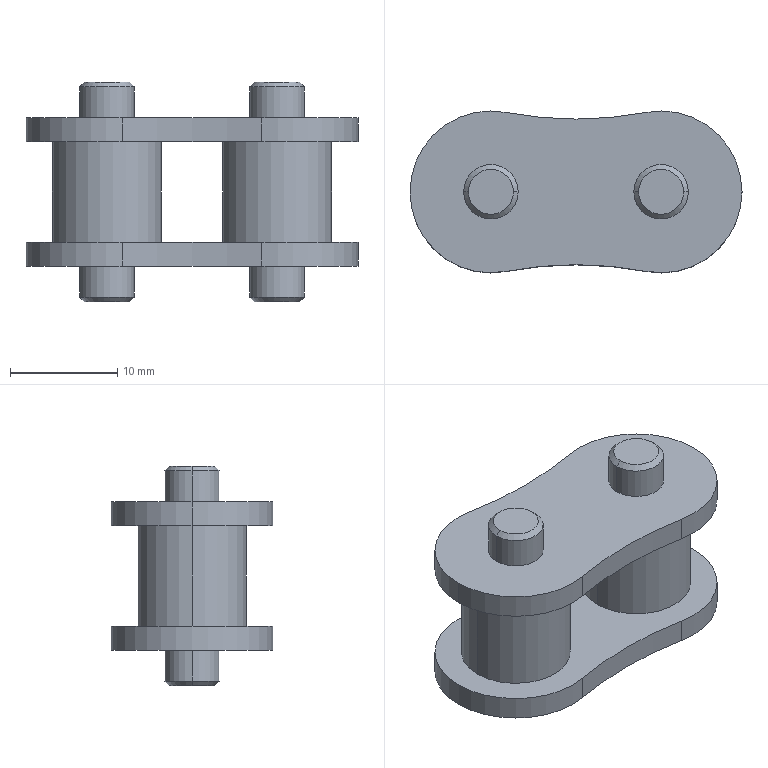Part | NX | features BREP 1 | 1 solid | 38 faces | box 30.965 x 15.09 x 20.5 mm | volume 3582 mm3 | cylinder 22 | cone 8 | plane 8 | commonest cylinder face diameters 5.09 x8 15.09 x6 10.16 x4 69.169 x4
STEP:
#1=CARTESIAN_POINT('',(-10.039,0.,-10.25));
#2=VERTEX_POINT('',#1);
#3=CARTESIAN_POINT('',(-5.837,0.,-10.25));
#4=VERTEX_POINT('',#3);
#5=CARTESIAN_POINT('',(-7.938,0.,-10.25));
#6=DIRECTION('',(0.,0.,-1.));
#7=DIRECTION('',(-1.,0.,0.));
#8=AXIS2_PLACEMENT_3D('',#5,#6,#7);
#9=CIRCLE('',#8,2.101);
#10=EDGE_CURVE('',#2,#4,#9,.T.);
#11=ORIENTED_EDGE('',*,*,#10,.F.);
#12=CARTESIAN_POINT('',(-10.482,0.,-9.806));
#13=VERTEX_POINT('',#12);
#14=CARTESIAN_POINT('',(-10.482,0.,-9.806));
#15=DIRECTION('',(-0.7071,0.,0.7071));
#16=VECTOR('',#15,1000.);
#17=LINE('',#14,#16);
#18=EDGE_CURVE('',#13,#2,#17,.F.);
#19=ORIENTED_EDGE('',*,*,#18,.F.);
#20=CARTESIAN_POINT('',(-5.393,0.,-9.806));
#21=VERTEX_POINT('',#20);
#22=CARTESIAN_POINT('',(-7.938,0.,-9.806));
#23=DIRECTION('',(0.,0.,1.));
#24=DIRECTION('',(-1.,0.,0.));
#25=AXIS2_PLACEMENT_3D('',#22,#23,#24);
#26=CIRCLE('',#25,2.545);
#27=EDGE_CURVE('',#21,#13,#26,.T.);
#28=ORIENTED_EDGE('',*,*,#27,.F.);
#29=CARTESIAN_POINT('',(-5.393,0.,-9.806));
#30=DIRECTION('',(0.7071,0.,0.7071));
#31=VECTOR('',#30,1000.);
#32=LINE('',#29,#31);
#33=EDGE_CURVE('',#21,#4,#32,.F.);
#34=ORIENTED_EDGE('',*,*,#33,.T.);
#35=EDGE_LOOP('',(#11,#19,#28,#34));
#36=FACE_BOUND('',#35,.T.);
#37=CARTESIAN_POINT('',(-7.938,0.,-9.806));
#38=DIRECTION('',(0.,0.,1.));
#39=DIRECTION('',(1.,0.,0.));
#40=AXIS2_PLACEMENT_3D('',#37,#38,#39);
#41=CONICAL_SURFACE('',#40,2.545,0.7854);
#42=ADVANCED_FACE('',(#36),#41,.T.);
#43=CARTESIAN_POINT('',(5.837,0.,-10.25));
#44=VERTEX_POINT('',#43);
#45=CARTESIAN_POINT('',(10.039,0.,-10.25));
#46=VERTEX_POINT('',#45);
#47=CARTESIAN_POINT('',(7.938,0.,-10.25));
#48=DIRECTION('',(0.,0.,-1.));
#49=DIRECTION('',(-1.,0.,0.));
#50=AXIS2_PLACEMENT_3D('',#47,#48,#49);
#51=CIRCLE('',#50,2.101);
#52=EDGE_CURVE('',#44,#46,#51,.T.);
#53=ORIENTED_EDGE('',*,*,#52,.F.);
#54=CARTESIAN_POINT('',(5.393,0.,-9.806));
#55=VERTEX_POINT('',#54);
#56=CARTESIAN_POINT('',(5.393,0.,-9.806));
#57=DIRECTION('',(-0.7071,0.,0.7071));
#58=VECTOR('',#57,1000.);
#59=LINE('',#56,#58);
#60=EDGE_CURVE('',#55,#44,#59,.F.);
#61=ORIENTED_EDGE('',*,*,#60,.F.);
#62=CARTESIAN_POINT('',(10.482,0.,-9.806));
#63=VERTEX_POINT('',#62);
#64=CARTESIAN_POINT('',(7.938,0.,-9.806));
#65=DIRECTION('',(0.,0.,1.));
#66=DIRECTION('',(-1.,0.,0.));
#67=AXIS2_PLACEMENT_3D('',#64,#65,#66);
#68=CIRCLE('',#67,2.545);
#69=EDGE_CURVE('',#63,#55,#68,.T.);
#70=ORIENTED_EDGE('',*,*,#69,.F.);
#71=CARTESIAN_POINT('',(10.482,0.,-9.806));
#72=DIRECTION('',(0.7071,0.,0.7071));
#73=VECTOR('',#72,1000.);
#74=LINE('',#71,#73);
#75=EDGE_CURVE('',#63,#46,#74,.F.);
#76=ORIENTED_EDGE('',*,*,#75,.T.);
#77=EDGE_LOOP('',(#53,#61,#70,#76));
#78=FACE_BOUND('',#77,.T.);
#79=CARTESIAN_POINT('',(7.938,0.,-9.806));
#80=DIRECTION('',(0.,0.,1.));
#81=DIRECTION('',(1.,0.,0.));
#82=AXIS2_PLACEMENT_3D('',#79,#80,#81);
#83=CONICAL_SURFACE('',#82,2.545,0.7854);
#84=ADVANCED_FACE('',(#78),#83,.T.);
#85=ORIENTED_EDGE('',*,*,#27,.T.);
#86=CARTESIAN_POINT('',(-10.482,0.,-6.92));
#87=VERTEX_POINT('',#86);
#88=CARTESIAN_POINT('',(-10.482,0.,-10.25));
#89=DIRECTION('',(0.,0.,1.));
#90=VECTOR('',#89,1000.);
#91=LINE('',#88,#90);
#92=EDGE_CURVE('',#87,#13,#91,.F.);
#93=ORIENTED_EDGE('',*,*,#92,.F.);
#94=CARTESIAN_POINT('',(-5.393,0.,-6.92));
#95=VERTEX_POINT('',#94);
#96=CARTESIAN_POINT('',(-7.938,0.,-6.92));
#97=DIRECTION('',(0.,0.,-1.));
#98=DIRECTION('',(-1.,0.,0.));
#99=AXIS2_PLACEMENT_3D('',#96,#97,#98);
#100=CIRCLE('',#99,2.545);
#101=EDGE_CURVE('',#87,#95,#100,.T.);
#102=ORIENTED_EDGE('',*,*,#101,.T.);
#103=CARTESIAN_POINT('',(-5.393,0.,-10.25));
#104=DIRECTION('',(0.,0.,1.));
#105=VECTOR('',#104,1000.);
#106=LINE('',#103,#105);
#107=EDGE_CURVE('',#95,#21,#106,.F.);
#108=ORIENTED_EDGE('',*,*,#107,.T.);
#109=EDGE_LOOP('',(#85,#93,#102,#108));
#110=FACE_BOUND('',#109,.T.);
#111=CARTESIAN_POINT('',(-7.938,0.,-10.25));
#112=DIRECTION('',(0.,0.,1.));
#113=DIRECTION('',(1.,0.,0.));
#114=AXIS2_PLACEMENT_3D('',#111,#112,#113);
#115=CYLINDRICAL_SURFACE('',#114,2.545);
#116=ADVANCED_FACE('',(#110),#115,.T.);
#117=ORIENTED_EDGE('',*,*,#69,.T.);
#118=CARTESIAN_POINT('',(5.393,0.,-6.92));
#119=VERTEX_POINT('',#118);
#120=CARTESIAN_POINT('',(5.393,0.,-10.25));
#121=DIRECTION('',(0.,0.,1.));
#122=VECTOR('',#121,1000.);
#123=LINE('',#120,#122);
#124=EDGE_CURVE('',#119,#55,#123,.F.);
#125=ORIENTED_EDGE('',*,*,#124,.F.);
#126=CARTESIAN_POINT('',(10.482,0.,-6.92));
#127=VERTEX_POINT('',#126);
#128=CARTESIAN_POINT('',(7.938,0.,-6.92));
#129=DIRECTION('',(0.,0.,-1.));
#130=DIRECTION('',(-1.,0.,0.));
#131=AXIS2_PLACEMENT_3D('',#128,#129,#130);
#132=CIRCLE('',#131,2.545);
#133=EDGE_CURVE('',#119,#127,#132,.T.);
#134=ORIENTED_EDGE('',*,*,#133,.T.);
#135=CARTESIAN_POINT('',(10.482,0.,-10.25));
#136=DIRECTION('',(0.,0.,1.));
#137=VECTOR('',#136,1000.);
#138=LINE('',#135,#137);
#139=EDGE_CURVE('',#127,#63,#138,.F.);
#140=ORIENTED_EDGE('',*,*,#139,.T.);
#141=EDGE_LOOP('',(#117,#125,#134,#140));
#142=FACE_BOUND('',#141,.T.);
#143=CARTESIAN_POINT('',(7.938,0.,-10.25));
#144=DIRECTION('',(0.,0.,1.));
#145=DIRECTION('',(1.,0.,0.));
#146=AXIS2_PLACEMENT_3D('',#143,#144,#145);
#147=CYLINDRICAL_SURFACE('',#146,2.545);
#148=ADVANCED_FACE('',(#142),#147,.T.);
#149=CARTESIAN_POINT('',(6.516,-7.41,-6.92));
#150=VERTEX_POINT('',#149);
#151=CARTESIAN_POINT('',(15.482,0.,-6.92));
#152=VERTEX_POINT('',#151);
#153=CARTESIAN_POINT('',(7.938,0.,-6.92));
#154=DIRECTION('',(0.,0.,1.));
#155=DIRECTION('',(1.,0.,0.));
#156=AXIS2_PLACEMENT_3D('',#153,#154,#155);
#157=CIRCLE('',#156,7.545);
#158=EDGE_CURVE('',#150,#152,#157,.T.);
#159=ORIENTED_EDGE('',*,*,#158,.T.);
#160=CARTESIAN_POINT('',(15.482,0.,-4.7));
#161=VERTEX_POINT('',#160);
#162=CARTESIAN_POINT('',(15.482,0.,-6.92));
#163=DIRECTION('',(0.,0.,1.));
#164=VECTOR('',#163,1000.);
#165=LINE('',#162,#164);
#166=EDGE_CURVE('',#152,#161,#165,.T.);
#167=ORIENTED_EDGE('',*,*,#166,.T.);
#168=CARTESIAN_POINT('',(6.516,-7.41,-4.7));
#169=VERTEX_POINT('',#168);
#170=CARTESIAN_POINT('',(7.938,0.,-4.7));
#171=DIRECTION('',(0.,0.,1.));
#172=DIRECTION('',(1.,0.,0.));
#173=AXIS2_PLACEMENT_3D('',#170,#171,#172);
#174=CIRCLE('',#173,7.545);
#175=EDGE_CURVE('',#169,#161,#174,.T.);
#176=ORIENTED_EDGE('',*,*,#175,.F.);
#177=CARTESIAN_POINT('',(6.516,-7.41,-6.92));
#178=DIRECTION('',(0.,0.,1.));
#179=VECTOR('',#178,1000.);
#180=LINE('',#177,#179);
#181=EDGE_CURVE('',#150,#169,#180,.T.);
#182=ORIENTED_EDGE('',*,*,#181,.F.);
#183=EDGE_LOOP('',(#159,#167,#176,#182));
#184=FACE_BOUND('',#183,.T.);
#185=CARTESIAN_POINT('',(7.938,0.,-6.92));
#186=DIRECTION('',(0.,0.,1.));
#187=DIRECTION('',(1.,0.,0.));
#188=AXIS2_PLACEMENT_3D('',#185,#186,#187);
#189=CYLINDRICAL_SURFACE('',#188,7.545);
#190=ADVANCED_FACE('',(#184),#189,.T.);
#191=CARTESIAN_POINT('',(-5.837,0.,10.25));
#192=VERTEX_POINT('',#191);
#193=CARTESIAN_POINT('',(-10.039,0.,10.25));
#194=VERTEX_POINT('',#193);
#195=CARTESIAN_POINT('',(-7.938,0.,10.25));
#196=DIRECTION('',(0.,0.,1.));
#197=DIRECTION('',(1.,0.,0.));
#198=AXIS2_PLACEMENT_3D('',#195,#196,#197);
#199=CIRCLE('',#198,2.101);
#200=EDGE_CURVE('',#192,#194,#199,.T.);
#201=ORIENTED_EDGE('',*,*,#200,.F.);
#202=CARTESIAN_POINT('',(-5.393,0.,9.806));
#203=VERTEX_POINT('',#202);
#204=CARTESIAN_POINT('',(-5.837,0.,10.25));
#205=DIRECTION('',(0.7071,0.,-0.7071));
#206=VECTOR('',#205,1000.);
#207=LINE('',#204,#206);
#208=EDGE_CURVE('',#192,#203,#207,.T.);
#209=ORIENTED_EDGE('',*,*,#208,.T.);
#210=CARTESIAN_POINT('',(-10.482,0.,9.806));
#211=VERTEX_POINT('',#210);
#212=CARTESIAN_POINT('',(-7.938,0.,9.806));
#213=DIRECTION('',(0.,0.,-1.));
#214=DIRECTION('',(1.,0.,0.));
#215=AXIS2_PLACEMENT_3D('',#212,#213,#214);
#216=CIRCLE('',#215,2.545);
#217=EDGE_CURVE('',#211,#203,#216,.T.);
#218=ORIENTED_EDGE('',*,*,#217,.F.);
#219=CARTESIAN_POINT('',(-10.039,0.,10.25));
#220=DIRECTION('',(-0.7071,0.,-0.7071));
#221=VECTOR('',#220,1000.);
#222=LINE('',#219,#221);
#223=EDGE_CURVE('',#194,#211,#222,.T.);
#224=ORIENTED_EDGE('',*,*,#223,.F.);
#225=EDGE_LOOP('',(#201,#209,#218,#224));
#226=FACE_BOUND('',#225,.T.);
#227=CARTESIAN_POINT('',(-7.938,0.,10.25));
#228=DIRECTION('',(0.,0.,-1.));
#229=DIRECTION('',(-1.,0.,0.));
#230=AXIS2_PLACEMENT_3D('',#227,#228,#229);
#231=CONICAL_SURFACE('',#230,2.101,0.7854);
#232=ADVANCED_FACE('',(#226),#231,.T.);
#233=CARTESIAN_POINT('',(10.039,0.,10.25));
#234=VERTEX_POINT('',#233);
#235=CARTESIAN_POINT('',(5.837,0.,10.25));
#236=VERTEX_POINT('',#235);
#237=CARTESIAN_POINT('',(7.938,0.,10.25));
#238=DIRECTION('',(0.,0.,1.));
#239=DIRECTION('',(1.,0.,0.));
#240=AXIS2_PLACEMENT_3D('',#237,#238,#239);
#241=CIRCLE('',#240,2.101);
#242=EDGE_CURVE('',#234,#236,#241,.T.);
#243=ORIENTED_EDGE('',*,*,#242,.F.);
#244=CARTESIAN_POINT('',(10.482,0.,9.806));
#245=VERTEX_POINT('',#244);
#246=CARTESIAN_POINT('',(10.039,0.,10.25));
#247=DIRECTION('',(0.7071,0.,-0.7071));
#248=VECTOR('',#247,1000.);
#249=LINE('',#246,#248);
#250=EDGE_CURVE('',#234,#245,#249,.T.);
#251=ORIENTED_EDGE('',*,*,#250,.T.);
#252=CARTESIAN_POINT('',(5.393,0.,9.806));
#253=VERTEX_POINT('',#252);
#254=CARTESIAN_POINT('',(7.938,0.,9.806));
#255=DIRECTION('',(0.,0.,-1.));
#256=DIRECTION('',(1.,0.,0.));
#257=AXIS2_PLACEMENT_3D('',#254,#255,#256);
#258=CIRCLE('',#257,2.545);
#259=EDGE_CURVE('',#253,#245,#258,.T.);
#260=ORIENTED_EDGE('',*,*,#259,.F.);
#261=CARTESIAN_POINT('',(5.837,0.,10.25));
#262=DIRECTION('',(-0.7071,0.,-0.7071));
#263=VECTOR('',#262,1000.);
#264=LINE('',#261,#263);
#265=EDGE_CURVE('',#236,#253,#264,.T.);
#266=ORIENTED_EDGE('',*,*,#265,.F.);
#267=EDGE_LOOP('',(#243,#251,#260,#266));
#268=FACE_BOUND('',#267,.T.);
#269=CARTESIAN_POINT('',(7.938,0.,10.25));
#270=DIRECTION('',(0.,0.,-1.));
#271=DIRECTION('',(-1.,0.,0.));
#272=AXIS2_PLACEMENT_3D('',#269,#270,#271);
#273=CONICAL_SURFACE('',#272,2.101,0.7854);
#274=ADVANCED_FACE('',(#268),#273,.T.);
#275=ORIENTED_EDGE('',*,*,#217,.T.);
#276=CARTESIAN_POINT('',(-5.393,0.,6.92));
#277=VERTEX_POINT('',#276);
#278=CARTESIAN_POINT('',(-5.393,0.,10.25));
#279=DIRECTION('',(0.,0.,-1.));
#280=VECTOR('',#279,1000.);
#281=LINE('',#278,#280);
#282=EDGE_CURVE('',#203,#277,#281,.T.);
#283=ORIENTED_EDGE('',*,*,#282,.T.);
#284=CARTESIAN_POINT('',(-10.482,0.,6.92));
#285=VERTEX_POINT('',#284);
#286=CARTESIAN_POINT('',(-7.938,0.,6.92));
#287=DIRECTION('',(0.,0.,1.));
#288=DIRECTION('',(1.,0.,0.));
#289=AXIS2_PLACEMENT_3D('',#286,#287,#288);
#290=CIRCLE('',#289,2.545);
#291=EDGE_CURVE('',#277,#285,#290,.T.);
#292=ORIENTED_EDGE('',*,*,#291,.T.);
#293=CARTESIAN_POINT('',(-10.482,0.,10.25));
#294=DIRECTION('',(0.,0.,-1.));
#295=VECTOR('',#294,1000.);
#296=LINE('',#293,#295);
#297=EDGE_CURVE('',#211,#285,#296,.T.);
#298=ORIENTED_EDGE('',*,*,#297,.F.);
#299=EDGE_LOOP('',(#275,#283,#292,#298));
#300=FACE_BOUND('',#299,.T.);
#301=CARTESIAN_POINT('',(-7.938,0.,10.25));
#302=DIRECTION('',(0.,0.,-1.));
#303=DIRECTION('',(-1.,0.,0.));
#304=AXIS2_PLACEMENT_3D('',#301,#302,#303);
#305=CYLINDRICAL_SURFACE('',#304,2.545);
#306=ADVANCED_FACE('',(#300),#305,.T.);
#307=ORIENTED_EDGE('',*,*,#259,.T.);
#308=CARTESIAN_POINT('',(10.482,0.,6.92));
#309=VERTEX_POINT('',#308);
#310=CARTESIAN_POINT('',(10.482,0.,10.25));
#311=DIRECTION('',(0.,0.,-1.));
#312=VECTOR('',#311,1000.);
#313=LINE('',#310,#312);
#314=EDGE_CURVE('',#245,#309,#313,.T.);
#315=ORIENTED_EDGE('',*,*,#314,.T.);
#316=CARTESIAN_POINT('',(5.393,0.,6.92));
#317=VERTEX_POINT('',#316);
#318=CARTESIAN_POINT('',(7.938,0.,6.92));
#319=DIRECTION('',(0.,0.,1.));
#320=DIRECTION('',(1.,0.,0.));
#321=AXIS2_PLACEMENT_3D('',#318,#319,#320);
#322=CIRCLE('',#321,2.545);
#323=EDGE_CURVE('',#309,#317,#322,.T.);
#324=ORIENTED_EDGE('',*,*,#323,.T.);
#325=CARTESIAN_POINT('',(5.393,0.,10.25));
#326=DIRECTION('',(0.,0.,-1.));
#327=VECTOR('',#326,1000.);
#328=LINE('',#325,#327);
#329=EDGE_CURVE('',#253,#317,#328,.T.);
#330=ORIENTED_EDGE('',*,*,#329,.F.);
#331=EDGE_LOOP('',(#307,#315,#324,#330));
#332=FACE_BOUND('',#331,.T.);
#333=CARTESIAN_POINT('',(7.938,0.,10.25));
#334=DIRECTION('',(0.,0.,-1.));
#335=DIRECTION('',(-1.,0.,0.));
#336=AXIS2_PLACEMENT_3D('',#333,#334,#335);
#337=CYLINDRICAL_SURFACE('',#336,2.545);
#338=ADVANCED_FACE('',(#332),#337,.T.);
#339=CARTESIAN_POINT('',(-13.018,0.,4.7));
#340=VERTEX_POINT('',#339);
#341=CARTESIAN_POINT('',(-2.857,0.,4.7));
#342=VERTEX_POINT('',#341);
#343=CARTESIAN_POINT('',(-7.938,0.,4.7));
#344=DIRECTION('',(0.,0.,-1.));
#345=DIRECTION('',(1.,0.,0.));
#346=AXIS2_PLACEMENT_3D('',#343,#344,#345);
#347=CIRCLE('',#346,5.08);
#348=EDGE_CURVE('',#340,#342,#347,.T.);
#349=ORIENTED_EDGE('',*,*,#348,.T.);
#350=CARTESIAN_POINT('',(-2.857,0.,-4.7));
#351=VERTEX_POINT('',#350);
#352=CARTESIAN_POINT('',(-2.857,0.,4.7));
#353=DIRECTION('',(0.,0.,-1.));
#354=VECTOR('',#353,1000.);
#355=LINE('',#352,#354);
#356=EDGE_CURVE('',#342,#351,#355,.T.);
#357=ORIENTED_EDGE('',*,*,#356,.T.);
#358=CARTESIAN_POINT('',(-13.018,0.,-4.7));
#359=VERTEX_POINT('',#358);
#360=CARTESIAN_POINT('',(-7.938,0.,-4.7));
#361=DIRECTION('',(0.,0.,-1.));
#362=DIRECTION('',(-1.,0.,0.));
#363=AXIS2_PLACEMENT_3D('',#360,#361,#362);
#364=CIRCLE('',#363,5.08);
#365=EDGE_CURVE('',#359,#351,#364,.T.);
#366=ORIENTED_EDGE('',*,*,#365,.F.);
#367=CARTESIAN_POINT('',(-13.018,0.,4.7));
#368=DIRECTION('',(0.,0.,-1.));
#369=VECTOR('',#368,1000.);
#370=LINE('',#367,#369);
#371=EDGE_CURVE('',#340,#359,#370,.T.);
#372=ORIENTED_EDGE('',*,*,#371,.F.);
#373=EDGE_LOOP('',(#349,#357,#366,#372));
#374=FACE_BOUND('',#373,.T.);
#375=CARTESIAN_POINT('',(-7.938,0.,4.7));
#376=DIRECTION('',(0.,0.,-1.));
#377=DIRECTION('',(-1.,0.,0.));
#378=AXIS2_PLACEMENT_3D('',#375,#376,#377);
#379=CYLINDRICAL_SURFACE('',#378,5.08);
#380=ADVANCED_FACE('',(#374),#379,.T.);
#381=CARTESIAN_POINT('',(-15.482,0.,6.92));
#382=VERTEX_POINT('',#381);
#383=CARTESIAN_POINT('',(-6.516,-7.41,6.92));
#384=VERTEX_POINT('',#383);
#385=CARTESIAN_POINT('',(-7.938,0.,6.92));
#386=DIRECTION('',(0.,0.,1.));
#387=DIRECTION('',(1.,0.,0.));
#388=AXIS2_PLACEMENT_3D('',#385,#386,#387);
#389=CIRCLE('',#388,7.545);
#390=EDGE_CURVE('',#382,#384,#389,.T.);
#391=ORIENTED_EDGE('',*,*,#390,.F.);
#392=CARTESIAN_POINT('',(-15.482,0.,4.7));
#393=VERTEX_POINT('',#392);
#394=CARTESIAN_POINT('',(-15.482,0.,6.92));
#395=DIRECTION('',(0.,0.,-1.));
#396=VECTOR('',#395,1000.);
#397=LINE('',#394,#396);
#398=EDGE_CURVE('',#382,#393,#397,.T.);
#399=ORIENTED_EDGE('',*,*,#398,.T.);
#400=CARTESIAN_POINT('',(-6.516,-7.41,4.7));
#401=VERTEX_POINT('',#400);
#402=CARTESIAN_POINT('',(-7.938,0.,4.7));
#403=DIRECTION('',(0.,0.,1.));
#404=DIRECTION('',(1.,0.,0.));
#405=AXIS2_PLACEMENT_3D('',#402,#403,#404);
#406=CIRCLE('',#405,7.545);
#407=EDGE_CURVE('',#393,#401,#406,.T.);
#408=ORIENTED_EDGE('',*,*,#407,.T.);
#409=CARTESIAN_POINT('',(-6.516,-7.41,6.92));
#410=DIRECTION('',(0.,0.,-1.));
#411=VECTOR('',#410,1000.);
#412=LINE('',#409,#411);
#413=EDGE_CURVE('',#384,#401,#412,.T.);
#414=ORIENTED_EDGE('',*,*,#413,.F.);
#415=EDGE_LOOP('',(#391,#399,#408,#414));
#416=FACE_BOUND('',#415,.T.);
#417=CARTESIAN_POINT('',(-7.938,0.,6.92));
#418=DIRECTION('',(0.,0.,-1.));
#419=DIRECTION('',(-1.,0.,0.));
#420=AXIS2_PLACEMENT_3D('',#417,#418,#419);
#421=CYLINDRICAL_SURFACE('',#420,7.545);
#422=ADVANCED_FACE('',(#416),#421,.T.);
#423=CARTESIAN_POINT('',(13.018,0.,4.7));
#424=VERTEX_POINT('',#423);
#425=CARTESIAN_POINT('',(2.857,0.,4.7));
#426=VERTEX_POINT('',#425);
#427=CARTESIAN_POINT('',(7.938,0.,4.7));
#428=DIRECTION('',(0.,0.,1.));
#429=DIRECTION('',(1.,0.,0.));
#430=AXIS2_PLACEMENT_3D('',#427,#428,#429);
#431=CIRCLE('',#430,5.08);
#432=EDGE_CURVE('',#424,#426,#431,.T.);
#433=ORIENTED_EDGE('',*,*,#432,.F.);
#434=CARTESIAN_POINT('',(13.018,0.,-4.7));
#435=VERTEX_POINT('',#434);
#436=CARTESIAN_POINT('',(13.018,0.,4.7));
#437=DIRECTION('',(0.,0.,-1.));
#438=VECTOR('',#437,1000.);
#439=LINE('',#436,#438);
#440=EDGE_CURVE('',#424,#435,#439,.T.);
#441=ORIENTED_EDGE('',*,*,#440,.T.);
#442=CARTESIAN_POINT('',(2.857,0.,-4.7));
#443=VERTEX_POINT('',#442);
#444=CARTESIAN_POINT('',(7.938,0.,-4.7));
#445=DIRECTION('',(0.,0.,-1.));
#446=DIRECTION('',(-1.,0.,0.));
#447=AXIS2_PLACEMENT_3D('',#444,#445,#446);
#448=CIRCLE('',#447,5.08);
#449=EDGE_CURVE('',#443,#435,#448,.T.);
#450=ORIENTED_EDGE('',*,*,#449,.F.);
#451=CARTESIAN_POINT('',(2.857,0.,4.7));
#452=DIRECTION('',(0.,0.,-1.));
#453=VECTOR('',#452,1000.);
#454=LINE('',#451,#453);
#455=EDGE_CURVE('',#426,#443,#454,.T.);
#456=ORIENTED_EDGE('',*,*,#455,.F.);
#457=EDGE_LOOP('',(#433,#441,#450,#456));
#458=FACE_BOUND('',#457,.T.);
#459=CARTESIAN_POINT('',(7.938,0.,4.7));
#460=DIRECTION('',(0.,0.,-1.));
#461=DIRECTION('',(-1.,0.,0.));
#462=AXIS2_PLACEMENT_3D('',#459,#460,#461);
#463=CYLINDRICAL_SURFACE('',#462,5.08);
#464=ADVANCED_FACE('',(#458),#463,.T.);
#465=CARTESIAN_POINT('',(6.516,-7.41,6.92));
#466=VERTEX_POINT('',#465);
#467=CARTESIAN_POINT('',(0.,-41.375,6.92));
#468=DIRECTION('',(0.,0.,-1.));
#469=DIRECTION('',(1.,0.,0.));
#470=AXIS2_PLACEMENT_3D('',#467,#468,#469);
#471=CIRCLE('',#470,34.584);
#472=EDGE_CURVE('',#384,#466,#471,.T.);
#473=ORIENTED_EDGE('',*,*,#472,.T.);
#474=CARTESIAN_POINT('',(6.516,7.41,6.92));
#475=VERTEX_POINT('',#474);
#476=CARTESIAN_POINT('',(7.938,0.,6.92));
#477=DIRECTION('',(0.,0.,1.));
#478=DIRECTION('',(1.,0.,0.));
#479=AXIS2_PLACEMENT_3D('',#476,#477,#478);
#480=CIRCLE('',#479,7.545);
#481=EDGE_CURVE('',#466,#475,#480,.T.);
#482=ORIENTED_EDGE('',*,*,#481,.T.);
#483=CARTESIAN_POINT('',(-6.516,7.41,6.92));
#484=VERTEX_POINT('',#483);
#485=CARTESIAN_POINT('',(0.,41.375,6.92));
#486=DIRECTION('',(0.,0.,-1.));
#487=DIRECTION('',(1.,0.,0.));
#488=AXIS2_PLACEMENT_3D('',#485,#486,#487);
#489=CIRCLE('',#488,34.584);
#490=EDGE_CURVE('',#475,#484,#489,.T.);
#491=ORIENTED_EDGE('',*,*,#490,.T.);
#492=CARTESIAN_POINT('',(-7.938,0.,6.92));
#493=DIRECTION('',(0.,0.,1.));
#494=DIRECTION('',(1.,0.,0.));
#495=AXIS2_PLACEMENT_3D('',#492,#493,#494);
#496=CIRCLE('',#495,7.545);
#497=EDGE_CURVE('',#484,#382,#496,.T.);
#498=ORIENTED_EDGE('',*,*,#497,.T.);
#499=ORIENTED_EDGE('',*,*,#390,.T.);
#500=EDGE_LOOP('',(#473,#482,#491,#498,#499));
#501=FACE_BOUND('',#500,.T.);
#502=CARTESIAN_POINT('',(7.938,0.,6.92));
#503=DIRECTION('',(0.,0.,1.));
#504=DIRECTION('',(1.,0.,0.));
#505=AXIS2_PLACEMENT_3D('',#502,#503,#504);
#506=CIRCLE('',#505,2.545);
#507=EDGE_CURVE('',#317,#309,#506,.T.);
#508=ORIENTED_EDGE('',*,*,#507,.F.);
#509=ORIENTED_EDGE('',*,*,#323,.F.);
#510=EDGE_LOOP('',(#508,#509));
#511=FACE_BOUND('',#510,.T.);
#512=CARTESIAN_POINT('',(-7.938,0.,6.92));
#513=DIRECTION('',(0.,0.,1.));
#514=DIRECTION('',(1.,0.,0.));
#515=AXIS2_PLACEMENT_3D('',#512,#513,#514);
#516=CIRCLE('',#515,2.545);
#517=EDGE_CURVE('',#285,#277,#516,.T.);
#518=ORIENTED_EDGE('',*,*,#517,.F.);
#519=ORIENTED_EDGE('',*,*,#291,.F.);
#520=EDGE_LOOP('',(#518,#519));
#521=FACE_BOUND('',#520,.T.);
#522=CARTESIAN_POINT('',(-3.969,-20.687,6.92));
#523=DIRECTION('',(0.,0.,1.));
#524=DIRECTION('',(1.,0.,0.));
#525=AXIS2_PLACEMENT_3D('',#522,#523,#524);
#526=PLANE('',#525);
#527=ADVANCED_FACE('',(#501,#511,#521),#526,.T.);
#528=CARTESIAN_POINT('',(6.516,-7.41,4.7));
#529=VERTEX_POINT('',#528);
#530=CARTESIAN_POINT('',(0.,-41.375,4.7));
#531=DIRECTION('',(0.,0.,-1.));
#532=DIRECTION('',(1.,0.,0.));
#533=AXIS2_PLACEMENT_3D('',#530,#531,#532);
#534=CIRCLE('',#533,34.584);
#535=EDGE_CURVE('',#401,#529,#534,.T.);
#536=ORIENTED_EDGE('',*,*,#535,.F.);
#537=ORIENTED_EDGE('',*,*,#407,.F.);
#538=CARTESIAN_POINT('',(-6.516,7.41,4.7));
#539=VERTEX_POINT('',#538);
#540=CARTESIAN_POINT('',(-7.938,0.,4.7));
#541=DIRECTION('',(0.,0.,1.));
#542=DIRECTION('',(1.,0.,0.));
#543=AXIS2_PLACEMENT_3D('',#540,#541,#542);
#544=CIRCLE('',#543,7.545);
#545=EDGE_CURVE('',#539,#393,#544,.T.);
#546=ORIENTED_EDGE('',*,*,#545,.F.);
#547=CARTESIAN_POINT('',(6.516,7.41,4.7));
#548=VERTEX_POINT('',#547);
#549=CARTESIAN_POINT('',(0.,41.375,4.7));
#550=DIRECTION('',(0.,0.,-1.));
#551=DIRECTION('',(1.,0.,0.));
#552=AXIS2_PLACEMENT_3D('',#549,#550,#551);
#553=CIRCLE('',#552,34.584);
#554=EDGE_CURVE('',#548,#539,#553,.T.);
#555=ORIENTED_EDGE('',*,*,#554,.F.);
#556=CARTESIAN_POINT('',(7.938,0.,4.7));
#557=DIRECTION('',(0.,0.,1.));
#558=DIRECTION('',(1.,0.,0.));
#559=AXIS2_PLACEMENT_3D('',#556,#557,#558);
#560=CIRCLE('',#559,7.545);
#561=EDGE_CURVE('',#529,#548,#560,.T.);
#562=ORIENTED_EDGE('',*,*,#561,.F.);
#563=EDGE_LOOP('',(#536,#537,#546,#555,#562));
#564=FACE_BOUND('',#563,.T.);
#565=CARTESIAN_POINT('',(7.938,0.,4.7));
#566=DIRECTION('',(0.,0.,1.));
#567=DIRECTION('',(1.,0.,0.));
#568=AXIS2_PLACEMENT_3D('',#565,#566,#567);
#569=CIRCLE('',#568,5.08);
#570=EDGE_CURVE('',#426,#424,#569,.T.);
#571=ORIENTED_EDGE('',*,*,#570,.T.);
#572=ORIENTED_EDGE('',*,*,#432,.T.);
#573=EDGE_LOOP('',(#571,#572));
#574=FACE_BOUND('',#573,.T.);
#575=ORIENTED_EDGE('',*,*,#348,.F.);
#576=CARTESIAN_POINT('',(-7.938,0.,4.7));
#577=DIRECTION('',(0.,0.,-1.));
#578=DIRECTION('',(1.,0.,0.));
#579=AXIS2_PLACEMENT_3D('',#576,#577,#578);
#580=CIRCLE('',#579,5.08);
#581=EDGE_CURVE('',#342,#340,#580,.T.);
#582=ORIENTED_EDGE('',*,*,#581,.F.);
#583=EDGE_LOOP('',(#575,#582));
#584=FACE_BOUND('',#583,.T.);
#585=CARTESIAN_POINT('',(-3.969,-20.687,4.7));
#586=DIRECTION('',(0.,0.,1.));
#587=DIRECTION('',(1.,0.,0.));
#588=AXIS2_PLACEMENT_3D('',#585,#586,#587);
#589=PLANE('',#588);
#590=ADVANCED_FACE('',(#564,#574,#584),#589,.F.);
#591=ORIENTED_EDGE('',*,*,#440,.F.);
#592=ORIENTED_EDGE('',*,*,#570,.F.);
#593=ORIENTED_EDGE('',*,*,#455,.T.);
#594=CARTESIAN_POINT('',(7.938,0.,-4.7));
#595=DIRECTION('',(0.,0.,-1.));
#596=DIRECTION('',(-1.,0.,0.));
#597=AXIS2_PLACEMENT_3D('',#594,#595,#596);
#598=CIRCLE('',#597,5.08);
#599=EDGE_CURVE('',#435,#443,#598,.T.);
#600=ORIENTED_EDGE('',*,*,#599,.F.);
#601=EDGE_LOOP('',(#591,#592,#593,#600));
#602=FACE_BOUND('',#601,.T.);
#603=CARTESIAN_POINT('',(7.938,0.,4.7));
#604=DIRECTION('',(0.,0.,-1.));
#605=DIRECTION('',(-1.,0.,0.));
#606=AXIS2_PLACEMENT_3D('',#603,#604,#605);
#607=CYLINDRICAL_SURFACE('',#606,5.08);
#608=ADVANCED_FACE('',(#602),#607,.T.);
#609=ORIENTED_EDGE('',*,*,#535,.T.);
#610=CARTESIAN_POINT('',(6.516,-7.41,6.92));
#611=DIRECTION('',(0.,0.,-1.));
#612=VECTOR('',#611,1000.);
#613=LINE('',#610,#612);
#614=EDGE_CURVE('',#466,#529,#613,.T.);
#615=ORIENTED_EDGE('',*,*,#614,.F.);
#616=ORIENTED_EDGE('',*,*,#472,.F.);
#617=ORIENTED_EDGE('',*,*,#413,.T.);
#618=EDGE_LOOP('',(#609,#615,#616,#617));
#619=FACE_BOUND('',#618,.T.);
#620=CARTESIAN_POINT('',(0.,-41.375,6.92));
#621=DIRECTION('',(0.,0.,-1.));
#622=DIRECTION('',(-1.,0.,0.));
#623=AXIS2_PLACEMENT_3D('',#620,#621,#622);
#624=CYLINDRICAL_SURFACE('',#623,34.584);
#625=ADVANCED_FACE('',(#619),#624,.F.);
#626=ORIENTED_EDGE('',*,*,#561,.T.);
#627=CARTESIAN_POINT('',(6.516,7.41,6.92));
#628=DIRECTION('',(0.,0.,-1.));
#629=VECTOR('',#628,1000.);
#630=LINE('',#627,#629);
#631=EDGE_CURVE('',#475,#548,#630,.T.);
#632=ORIENTED_EDGE('',*,*,#631,.F.);
#633=ORIENTED_EDGE('',*,*,#481,.F.);
#634=ORIENTED_EDGE('',*,*,#614,.T.);
#635=EDGE_LOOP('',(#626,#632,#633,#634));
#636=FACE_BOUND('',#635,.T.);
#637=CARTESIAN_POINT('',(7.938,0.,6.92));
#638=DIRECTION('',(0.,0.,-1.));
#639=DIRECTION('',(-1.,0.,0.));
#640=AXIS2_PLACEMENT_3D('',#637,#638,#639);
#641=CYLINDRICAL_SURFACE('',#640,7.545);
#642=ADVANCED_FACE('',(#636),#641,.T.);
#643=ORIENTED_EDGE('',*,*,#554,.T.);
#644=CARTESIAN_POINT('',(-6.516,7.41,6.92));
#645=DIRECTION('',(0.,0.,-1.));
#646=VECTOR('',#645,1000.);
#647=LINE('',#644,#646);
#648=EDGE_CURVE('',#484,#539,#647,.T.);
#649=ORIENTED_EDGE('',*,*,#648,.F.);
#650=ORIENTED_EDGE('',*,*,#490,.F.);
#651=ORIENTED_EDGE('',*,*,#631,.T.);
#652=EDGE_LOOP('',(#643,#649,#650,#651));
#653=FACE_BOUND('',#652,.T.);
#654=CARTESIAN_POINT('',(0.,41.375,6.92));
#655=DIRECTION('',(0.,0.,-1.));
#656=DIRECTION('',(-1.,0.,0.));
#657=AXIS2_PLACEMENT_3D('',#654,#655,#656);
#658=CYLINDRICAL_SURFACE('',#657,34.584);
#659=ADVANCED_FACE('',(#653),#658,.F.);
#660=ORIENTED_EDGE('',*,*,#398,.F.);
#661=ORIENTED_EDGE('',*,*,#497,.F.);
#662=ORIENTED_EDGE('',*,*,#648,.T.);
#663=ORIENTED_EDGE('',*,*,#545,.T.);
#664=EDGE_LOOP('',(#660,#661,#662,#663));
#665=FACE_BOUND('',#664,.T.);
#666=CARTESIAN_POINT('',(-7.938,0.,6.92));
#667=DIRECTION('',(0.,0.,-1.));
#668=DIRECTION('',(-1.,0.,0.));
#669=AXIS2_PLACEMENT_3D('',#666,#667,#668);
#670=CYLINDRICAL_SURFACE('',#669,7.545);
#671=ADVANCED_FACE('',(#665),#670,.T.);
#672=ORIENTED_EDGE('',*,*,#356,.F.);
#673=ORIENTED_EDGE('',*,*,#581,.T.);
#674=ORIENTED_EDGE('',*,*,#371,.T.);
#675=CARTESIAN_POINT('',(-7.938,0.,-4.7));
#676=DIRECTION('',(0.,0.,-1.));
#677=DIRECTION('',(-1.,0.,0.));
#678=AXIS2_PLACEMENT_3D('',#675,#676,#677);
#679=CIRCLE('',#678,5.08);
#680=EDGE_CURVE('',#351,#359,#679,.T.);
#681=ORIENTED_EDGE('',*,*,#680,.F.);
#682=EDGE_LOOP('',(#672,#673,#674,#681));
#683=FACE_BOUND('',#682,.T.);
#684=CARTESIAN_POINT('',(-7.938,0.,4.7));
#685=DIRECTION('',(0.,0.,-1.));
#686=DIRECTION('',(-1.,0.,0.));
#687=AXIS2_PLACEMENT_3D('',#684,#685,#686);
#688=CYLINDRICAL_SURFACE('',#687,5.08);
#689=ADVANCED_FACE('',(#683),#688,.T.);
#690=ORIENTED_EDGE('',*,*,#314,.F.);
#691=CARTESIAN_POINT('',(7.938,0.,9.806));
#692=DIRECTION('',(0.,0.,-1.));
#693=DIRECTION('',(1.,0.,0.));
#694=AXIS2_PLACEMENT_3D('',#691,#692,#693);
#695=CIRCLE('',#694,2.545);
#696=EDGE_CURVE('',#245,#253,#695,.T.);
#697=ORIENTED_EDGE('',*,*,#696,.T.);
#698=ORIENTED_EDGE('',*,*,#329,.T.);
#699=ORIENTED_EDGE('',*,*,#507,.T.);
#700=EDGE_LOOP('',(#690,#697,#698,#699));
#701=FACE_BOUND('',#700,.T.);
#702=CARTESIAN_POINT('',(7.938,0.,10.25));
#703=DIRECTION('',(0.,0.,-1.));
#704=DIRECTION('',(-1.,0.,0.));
#705=AXIS2_PLACEMENT_3D('',#702,#703,#704);
#706=CYLINDRICAL_SURFACE('',#705,2.545);
#707=ADVANCED_FACE('',(#701),#706,.T.);
#708=CARTESIAN_POINT('',(7.938,0.,10.25));
#709=DIRECTION('',(0.,0.,1.));
#710=DIRECTION('',(1.,0.,0.));
#711=AXIS2_PLACEMENT_3D('',#708,#709,#710);
#712=CIRCLE('',#711,2.101);
#713=EDGE_CURVE('',#236,#234,#712,.T.);
#714=ORIENTED_EDGE('',*,*,#713,.T.);
#715=ORIENTED_EDGE('',*,*,#242,.T.);
#716=EDGE_LOOP('',(#714,#715));
#717=FACE_BOUND('',#716,.T.);
#718=CARTESIAN_POINT('',(7.938,0.,10.25));
#719=DIRECTION('',(0.,0.,1.));
#720=DIRECTION('',(1.,0.,0.));
#721=AXIS2_PLACEMENT_3D('',#718,#719,#720);
#722=PLANE('',#721);
#723=ADVANCED_FACE('',(#717),#722,.T.);
#724=ORIENTED_EDGE('',*,*,#282,.F.);
#725=CARTESIAN_POINT('',(-7.938,0.,9.806));
#726=DIRECTION('',(0.,0.,-1.));
#727=DIRECTION('',(1.,0.,0.));
#728=AXIS2_PLACEMENT_3D('',#725,#726,#727);
#729=CIRCLE('',#728,2.545);
#730=EDGE_CURVE('',#203,#211,#729,.T.);
#731=ORIENTED_EDGE('',*,*,#730,.T.);
#732=ORIENTED_EDGE('',*,*,#297,.T.);
#733=ORIENTED_EDGE('',*,*,#517,.T.);
#734=EDGE_LOOP('',(#724,#731,#732,#733));
#735=FACE_BOUND('',#734,.T.);
#736=CARTESIAN_POINT('',(-7.938,0.,10.25));
#737=DIRECTION('',(0.,0.,-1.));
#738=DIRECTION('',(-1.,0.,0.));
#739=AXIS2_PLACEMENT_3D('',#736,#737,#738);
#740=CYLINDRICAL_SURFACE('',#739,2.545);
#741=ADVANCED_FACE('',(#735),#740,.T.);
#742=CARTESIAN_POINT('',(-7.938,0.,10.25));
#743=DIRECTION('',(0.,0.,1.));
#744=DIRECTION('',(1.,0.,0.));
#745=AXIS2_PLACEMENT_3D('',#742,#743,#744);
#746=CIRCLE('',#745,2.101);
#747=EDGE_CURVE('',#194,#192,#746,.T.);
#748=ORIENTED_EDGE('',*,*,#747,.T.);
#749=ORIENTED_EDGE('',*,*,#200,.T.);
#750=EDGE_LOOP('',(#748,#749));
#751=FACE_BOUND('',#750,.T.);
#752=CARTESIAN_POINT('',(-7.938,0.,10.25));
#753=DIRECTION('',(0.,0.,1.));
#754=DIRECTION('',(1.,0.,0.));
#755=AXIS2_PLACEMENT_3D('',#752,#753,#754);
#756=PLANE('',#755);
#757=ADVANCED_FACE('',(#751),#756,.T.);
#758=ORIENTED_EDGE('',*,*,#250,.F.);
#759=ORIENTED_EDGE('',*,*,#713,.F.);
#760=ORIENTED_EDGE('',*,*,#265,.T.);
#761=ORIENTED_EDGE('',*,*,#696,.F.);
#762=EDGE_LOOP('',(#758,#759,#760,#761));
#763=FACE_BOUND('',#762,.T.);
#764=CARTESIAN_POINT('',(7.938,0.,10.25));
#765=DIRECTION('',(0.,0.,-1.));
#766=DIRECTION('',(-1.,0.,0.));
#767=AXIS2_PLACEMENT_3D('',#764,#765,#766);
#768=CONICAL_SURFACE('',#767,2.101,0.7854);
#769=ADVANCED_FACE('',(#763),#768,.T.);
#770=ORIENTED_EDGE('',*,*,#208,.F.);
#771=ORIENTED_EDGE('',*,*,#747,.F.);
#772=ORIENTED_EDGE('',*,*,#223,.T.);
#773=ORIENTED_EDGE('',*,*,#730,.F.);
#774=EDGE_LOOP('',(#770,#771,#772,#773));
#775=FACE_BOUND('',#774,.T.);
#776=CARTESIAN_POINT('',(-7.938,0.,10.25));
#777=DIRECTION('',(0.,0.,-1.));
#778=DIRECTION('',(-1.,0.,0.));
#779=AXIS2_PLACEMENT_3D('',#776,#777,#778);
#780=CONICAL_SURFACE('',#779,2.101,0.7854);
#781=ADVANCED_FACE('',(#775),#780,.T.);
#782=CARTESIAN_POINT('',(-6.516,-7.41,-4.7));
#783=VERTEX_POINT('',#782);
#784=CARTESIAN_POINT('',(0.,-41.375,-4.7));
#785=DIRECTION('',(0.,0.,-1.));
#786=DIRECTION('',(1.,0.,0.));
#787=AXIS2_PLACEMENT_3D('',#784,#785,#786);
#788=CIRCLE('',#787,34.584);
#789=EDGE_CURVE('',#783,#169,#788,.T.);
#790=ORIENTED_EDGE('',*,*,#789,.T.);
#791=ORIENTED_EDGE('',*,*,#175,.T.);
#792=CARTESIAN_POINT('',(6.516,7.41,-4.7));
#793=VERTEX_POINT('',#792);
#794=CARTESIAN_POINT('',(7.938,0.,-4.7));
#795=DIRECTION('',(0.,0.,1.));
#796=DIRECTION('',(1.,0.,0.));
#797=AXIS2_PLACEMENT_3D('',#794,#795,#796);
#798=CIRCLE('',#797,7.545);
#799=EDGE_CURVE('',#161,#793,#798,.T.);
#800=ORIENTED_EDGE('',*,*,#799,.T.);
#801=CARTESIAN_POINT('',(-6.516,7.41,-4.7));
#802=VERTEX_POINT('',#801);
#803=CARTESIAN_POINT('',(0.,41.375,-4.7));
#804=DIRECTION('',(0.,0.,-1.));
#805=DIRECTION('',(1.,0.,0.));
#806=AXIS2_PLACEMENT_3D('',#803,#804,#805);
#807=CIRCLE('',#806,34.584);
#808=EDGE_CURVE('',#793,#802,#807,.T.);
#809=ORIENTED_EDGE('',*,*,#808,.T.);
#810=CARTESIAN_POINT('',(-7.938,0.,-4.7));
#811=DIRECTION('',(0.,0.,1.));
#812=DIRECTION('',(1.,0.,0.));
#813=AXIS2_PLACEMENT_3D('',#810,#811,#812);
#814=CIRCLE('',#813,7.545);
#815=EDGE_CURVE('',#802,#783,#814,.T.);
#816=ORIENTED_EDGE('',*,*,#815,.T.);
#817=EDGE_LOOP('',(#790,#791,#800,#809,#816));
#818=FACE_BOUND('',#817,.T.);
#819=ORIENTED_EDGE('',*,*,#365,.T.);
#820=ORIENTED_EDGE('',*,*,#680,.T.);
#821=EDGE_LOOP('',(#819,#820));
#822=FACE_BOUND('',#821,.T.);
#823=ORIENTED_EDGE('',*,*,#449,.T.);
#824=ORIENTED_EDGE('',*,*,#599,.T.);
#825=EDGE_LOOP('',(#823,#824));
#826=FACE_BOUND('',#825,.T.);
#827=CARTESIAN_POINT('',(-3.969,-20.687,-4.7));
#828=DIRECTION('',(0.,0.,-1.));
#829=DIRECTION('',(0.,-1.,0.));
#830=AXIS2_PLACEMENT_3D('',#827,#828,#829);
#831=PLANE('',#830);
#832=ADVANCED_FACE('',(#818,#822,#826),#831,.F.);
#833=ORIENTED_EDGE('',*,*,#789,.F.);
#834=CARTESIAN_POINT('',(-6.516,-7.41,-6.92));
#835=VERTEX_POINT('',#834);
#836=CARTESIAN_POINT('',(-6.516,-7.41,-6.92));
#837=DIRECTION('',(0.,0.,1.));
#838=VECTOR('',#837,1000.);
#839=LINE('',#836,#838);
#840=EDGE_CURVE('',#835,#783,#839,.T.);
#841=ORIENTED_EDGE('',*,*,#840,.F.);
#842=CARTESIAN_POINT('',(0.,-41.375,-6.92));
#843=DIRECTION('',(0.,0.,-1.));
#844=DIRECTION('',(1.,0.,0.));
#845=AXIS2_PLACEMENT_3D('',#842,#843,#844);
#846=CIRCLE('',#845,34.584);
#847=EDGE_CURVE('',#835,#150,#846,.T.);
#848=ORIENTED_EDGE('',*,*,#847,.T.);
#849=ORIENTED_EDGE('',*,*,#181,.T.);
#850=EDGE_LOOP('',(#833,#841,#848,#849));
#851=FACE_BOUND('',#850,.T.);
#852=CARTESIAN_POINT('',(0.,-41.375,-6.92));
#853=DIRECTION('',(0.,0.,1.));
#854=DIRECTION('',(1.,0.,0.));
#855=AXIS2_PLACEMENT_3D('',#852,#853,#854);
#856=CYLINDRICAL_SURFACE('',#855,34.584);
#857=ADVANCED_FACE('',(#851),#856,.F.);
#858=ORIENTED_EDGE('',*,*,#815,.F.);
#859=CARTESIAN_POINT('',(-6.516,7.41,-6.92));
#860=VERTEX_POINT('',#859);
#861=CARTESIAN_POINT('',(-6.516,7.41,-6.92));
#862=DIRECTION('',(0.,0.,1.));
#863=VECTOR('',#862,1000.);
#864=LINE('',#861,#863);
#865=EDGE_CURVE('',#860,#802,#864,.T.);
#866=ORIENTED_EDGE('',*,*,#865,.F.);
#867=CARTESIAN_POINT('',(-7.938,0.,-6.92));
#868=DIRECTION('',(0.,0.,1.));
#869=DIRECTION('',(1.,0.,0.));
#870=AXIS2_PLACEMENT_3D('',#867,#868,#869);
#871=CIRCLE('',#870,7.545);
#872=EDGE_CURVE('',#860,#835,#871,.T.);
#873=ORIENTED_EDGE('',*,*,#872,.T.);
#874=ORIENTED_EDGE('',*,*,#840,.T.);
#875=EDGE_LOOP('',(#858,#866,#873,#874));
#876=FACE_BOUND('',#875,.T.);
#877=CARTESIAN_POINT('',(-7.938,0.,-6.92));
#878=DIRECTION('',(0.,0.,1.));
#879=DIRECTION('',(1.,0.,0.));
#880=AXIS2_PLACEMENT_3D('',#877,#878,#879);
#881=CYLINDRICAL_SURFACE('',#880,7.545);
#882=ADVANCED_FACE('',(#876),#881,.T.);
#883=ORIENTED_EDGE('',*,*,#808,.F.);
#884=CARTESIAN_POINT('',(6.516,7.41,-6.92));
#885=VERTEX_POINT('',#884);
#886=CARTESIAN_POINT('',(6.516,7.41,-6.92));
#887=DIRECTION('',(0.,0.,1.));
#888=VECTOR('',#887,1000.);
#889=LINE('',#886,#888);
#890=EDGE_CURVE('',#885,#793,#889,.T.);
#891=ORIENTED_EDGE('',*,*,#890,.F.);
#892=CARTESIAN_POINT('',(0.,41.375,-6.92));
#893=DIRECTION('',(0.,0.,-1.));
#894=DIRECTION('',(1.,0.,0.));
#895=AXIS2_PLACEMENT_3D('',#892,#893,#894);
#896=CIRCLE('',#895,34.584);
#897=EDGE_CURVE('',#885,#860,#896,.T.);
#898=ORIENTED_EDGE('',*,*,#897,.T.);
#899=ORIENTED_EDGE('',*,*,#865,.T.);
#900=EDGE_LOOP('',(#883,#891,#898,#899));
#901=FACE_BOUND('',#900,.T.);
#902=CARTESIAN_POINT('',(0.,41.375,-6.92));
#903=DIRECTION('',(0.,0.,1.));
#904=DIRECTION('',(1.,0.,0.));
#905=AXIS2_PLACEMENT_3D('',#902,#903,#904);
#906=CYLINDRICAL_SURFACE('',#905,34.584);
#907=ADVANCED_FACE('',(#901),#906,.F.);
#908=ORIENTED_EDGE('',*,*,#166,.F.);
#909=CARTESIAN_POINT('',(7.938,0.,-6.92));
#910=DIRECTION('',(0.,0.,1.));
#911=DIRECTION('',(1.,0.,0.));
#912=AXIS2_PLACEMENT_3D('',#909,#910,#911);
#913=CIRCLE('',#912,7.545);
#914=EDGE_CURVE('',#152,#885,#913,.T.);
#915=ORIENTED_EDGE('',*,*,#914,.T.);
#916=ORIENTED_EDGE('',*,*,#890,.T.);
#917=ORIENTED_EDGE('',*,*,#799,.F.);
#918=EDGE_LOOP('',(#908,#915,#916,#917));
#919=FACE_BOUND('',#918,.T.);
#920=CARTESIAN_POINT('',(7.938,0.,-6.92));
#921=DIRECTION('',(0.,0.,1.));
#922=DIRECTION('',(1.,0.,0.));
#923=AXIS2_PLACEMENT_3D('',#920,#921,#922);
#924=CYLINDRICAL_SURFACE('',#923,7.545);
#925=ADVANCED_FACE('',(#919),#924,.T.);
#926=ORIENTED_EDGE('',*,*,#847,.F.);
#927=ORIENTED_EDGE('',*,*,#872,.F.);
#928=ORIENTED_EDGE('',*,*,#897,.F.);
#929=ORIENTED_EDGE('',*,*,#914,.F.);
#930=ORIENTED_EDGE('',*,*,#158,.F.);
#931=EDGE_LOOP('',(#926,#927,#928,#929,#930));
#932=FACE_BOUND('',#931,.T.);
#933=CARTESIAN_POINT('',(-7.938,0.,-6.92));
#934=DIRECTION('',(0.,0.,-1.));
#935=DIRECTION('',(-1.,0.,0.));
#936=AXIS2_PLACEMENT_3D('',#933,#934,#935);
#937=CIRCLE('',#936,2.545);
#938=EDGE_CURVE('',#95,#87,#937,.T.);
#939=ORIENTED_EDGE('',*,*,#938,.F.);
#940=ORIENTED_EDGE('',*,*,#101,.F.);
#941=EDGE_LOOP('',(#939,#940));
#942=FACE_BOUND('',#941,.T.);
#943=CARTESIAN_POINT('',(7.938,0.,-6.92));
#944=DIRECTION('',(0.,0.,-1.));
#945=DIRECTION('',(-1.,0.,0.));
#946=AXIS2_PLACEMENT_3D('',#943,#944,#945);
#947=CIRCLE('',#946,2.545);
#948=EDGE_CURVE('',#127,#119,#947,.T.);
#949=ORIENTED_EDGE('',*,*,#948,.F.);
#950=ORIENTED_EDGE('',*,*,#133,.F.);
#951=EDGE_LOOP('',(#949,#950));
#952=FACE_BOUND('',#951,.T.);
#953=CARTESIAN_POINT('',(-3.969,-20.687,-6.92));
#954=DIRECTION('',(0.,0.,-1.));
#955=DIRECTION('',(0.,-1.,0.));
#956=AXIS2_PLACEMENT_3D('',#953,#954,#955);
#957=PLANE('',#956);
#958=ADVANCED_FACE('',(#932,#942,#952),#957,.T.);
#959=ORIENTED_EDGE('',*,*,#124,.T.);
#960=CARTESIAN_POINT('',(7.938,0.,-9.806));
#961=DIRECTION('',(0.,0.,1.));
#962=DIRECTION('',(-1.,0.,0.));
#963=AXIS2_PLACEMENT_3D('',#960,#961,#962);
#964=CIRCLE('',#963,2.545);
#965=EDGE_CURVE('',#55,#63,#964,.T.);
#966=ORIENTED_EDGE('',*,*,#965,.T.);
#967=ORIENTED_EDGE('',*,*,#139,.F.);
#968=ORIENTED_EDGE('',*,*,#948,.T.);
#969=EDGE_LOOP('',(#959,#966,#967,#968));
#970=FACE_BOUND('',#969,.T.);
#971=CARTESIAN_POINT('',(7.938,0.,-10.25));
#972=DIRECTION('',(0.,0.,1.));
#973=DIRECTION('',(1.,0.,0.));
#974=AXIS2_PLACEMENT_3D('',#971,#972,#973);
#975=CYLINDRICAL_SURFACE('',#974,2.545);
#976=ADVANCED_FACE('',(#970),#975,.T.);
#977=CARTESIAN_POINT('',(7.938,0.,-10.25));
#978=DIRECTION('',(0.,0.,-1.));
#979=DIRECTION('',(-1.,0.,0.));
#980=AXIS2_PLACEMENT_3D('',#977,#978,#979);
#981=CIRCLE('',#980,2.101);
#982=EDGE_CURVE('',#46,#44,#981,.T.);
#983=ORIENTED_EDGE('',*,*,#982,.T.);
#984=ORIENTED_EDGE('',*,*,#52,.T.);
#985=EDGE_LOOP('',(#983,#984));
#986=FACE_BOUND('',#985,.T.);
#987=CARTESIAN_POINT('',(7.938,0.,-10.25));
#988=DIRECTION('',(0.,0.,-1.));
#989=DIRECTION('',(0.,-1.,0.));
#990=AXIS2_PLACEMENT_3D('',#987,#988,#989);
#991=PLANE('',#990);
#992=ADVANCED_FACE('',(#986),#991,.T.);
#993=ORIENTED_EDGE('',*,*,#92,.T.);
#994=CARTESIAN_POINT('',(-7.938,0.,-9.806));
#995=DIRECTION('',(0.,0.,1.));
#996=DIRECTION('',(-1.,0.,0.));
#997=AXIS2_PLACEMENT_3D('',#994,#995,#996);
#998=CIRCLE('',#997,2.545);
#999=EDGE_CURVE('',#13,#21,#998,.T.);
#1000=ORIENTED_EDGE('',*,*,#999,.T.);
#1001=ORIENTED_EDGE('',*,*,#107,.F.);
#1002=ORIENTED_EDGE('',*,*,#938,.T.);
#1003=EDGE_LOOP('',(#993,#1000,#1001,#1002));
#1004=FACE_BOUND('',#1003,.T.);
#1005=CARTESIAN_POINT('',(-7.938,0.,-10.25));
#1006=DIRECTION('',(0.,0.,1.));
#1007=DIRECTION('',(1.,0.,0.));
#1008=AXIS2_PLACEMENT_3D('',#1005,#1006,#1007);
#1009=CYLINDRICAL_SURFACE('',#1008,2.545);
#1010=ADVANCED_FACE('',(#1004),#1009,.T.);
#1011=CARTESIAN_POINT('',(-7.938,0.,-10.25));
#1012=DIRECTION('',(0.,0.,-1.));
#1013=DIRECTION('',(-1.,0.,0.));
#1014=AXIS2_PLACEMENT_3D('',#1011,#1012,#1013);
#1015=CIRCLE('',#1014,2.101);
#1016=EDGE_CURVE('',#4,#2,#1015,.T.);
#1017=ORIENTED_EDGE('',*,*,#1016,.T.);
#1018=ORIENTED_EDGE('',*,*,#10,.T.);
#1019=EDGE_LOOP('',(#1017,#1018));
#1020=FACE_BOUND('',#1019,.T.);
#1021=CARTESIAN_POINT('',(-7.938,0.,-10.25));
#1022=DIRECTION('',(0.,0.,-1.));
#1023=DIRECTION('',(0.,-1.,0.));
#1024=AXIS2_PLACEMENT_3D('',#1021,#1022,#1023);
#1025=PLANE('',#1024);
#1026=ADVANCED_FACE('',(#1020),#1025,.T.);
#1027=ORIENTED_EDGE('',*,*,#60,.T.);
#1028=ORIENTED_EDGE('',*,*,#982,.F.);
#1029=ORIENTED_EDGE('',*,*,#75,.F.);
#1030=ORIENTED_EDGE('',*,*,#965,.F.);
#1031=EDGE_LOOP('',(#1027,#1028,#1029,#1030));
#1032=FACE_BOUND('',#1031,.T.);
#1033=CARTESIAN_POINT('',(7.938,0.,-9.806));
#1034=DIRECTION('',(0.,0.,1.));
#1035=DIRECTION('',(1.,0.,0.));
#1036=AXIS2_PLACEMENT_3D('',#1033,#1034,#1035);
#1037=CONICAL_SURFACE('',#1036,2.545,0.7854);
#1038=ADVANCED_FACE('',(#1032),#1037,.T.);
#1039=ORIENTED_EDGE('',*,*,#18,.T.);
#1040=ORIENTED_EDGE('',*,*,#1016,.F.);
#1041=ORIENTED_EDGE('',*,*,#33,.F.);
#1042=ORIENTED_EDGE('',*,*,#999,.F.);
#1043=EDGE_LOOP('',(#1039,#1040,#1041,#1042));
#1044=FACE_BOUND('',#1043,.T.);
#1045=CARTESIAN_POINT('',(-7.938,0.,-9.806));
#1046=DIRECTION('',(0.,0.,1.));
#1047=DIRECTION('',(1.,0.,0.));
#1048=AXIS2_PLACEMENT_3D('',#1045,#1046,#1047);
#1049=CONICAL_SURFACE('',#1048,2.545,0.7854);
#1050=ADVANCED_FACE('',(#1044),#1049,.T.);
#1051=CLOSED_SHELL('',(#42,#84,#116,#148,#190,#232,#274,#306,#338,#380,#422,#464,#527,#590,#608,#625,#642,#659,#671,#689,#707,#723,#741,#757,#769,#781,#832,#857,#882,#907,#925,#958,#976,#992,#1010,#1026,#1038,#1050));
#1052=MANIFOLD_SOLID_BREP('',#1051);
#1053=(LENGTH_UNIT()NAMED_UNIT(*)SI_UNIT(.MILLI.,.METRE.));
#1054=UNCERTAINTY_MEASURE_WITH_UNIT(LENGTH_MEASURE(0.00001),#1053,'','');
#1055=(NAMED_UNIT(*)PLANE_ANGLE_UNIT()SI_UNIT($,.RADIAN.));
#1056=(NAMED_UNIT(*)SI_UNIT($,.STERADIAN.)SOLID_ANGLE_UNIT());
#1057=(GEOMETRIC_REPRESENTATION_CONTEXT(3)GLOBAL_UNCERTAINTY_ASSIGNED_CONTEXT((#1054))GLOBAL_UNIT_ASSIGNED_CONTEXT((#1053,#1055,#1056))REPRESENTATION_CONTEXT('',''));
#1058=ADVANCED_BREP_SHAPE_REPRESENTATION('',(#1052),#1057);